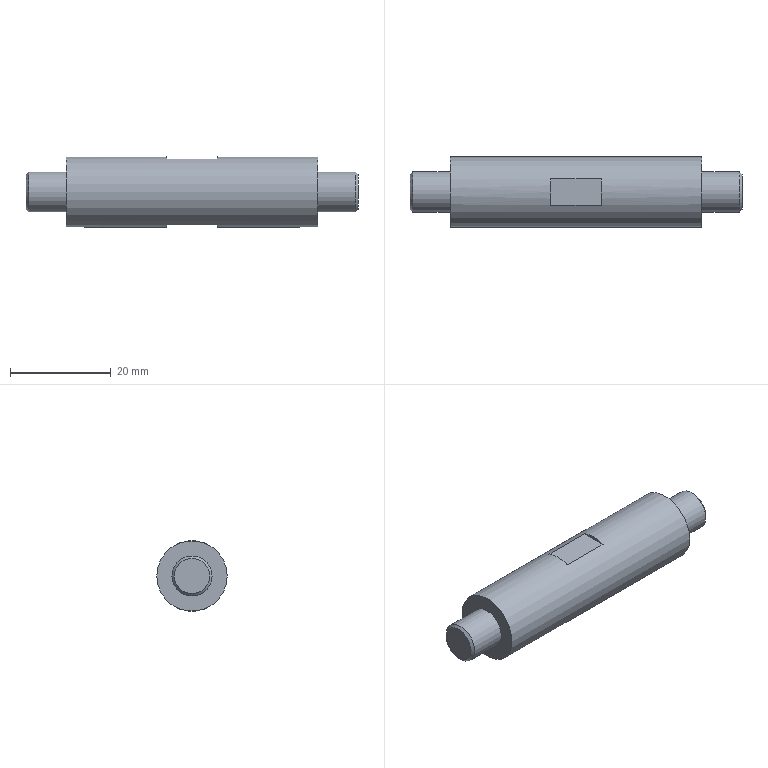Part | NX | features BREP 1 | 1 solid | 15 faces | box 66 x 14 x 14 mm | volume 8460 mm3 | plane 10 | cylinder 3 | cone 2 | commonest cylinder face diameters 8 x2 14 x1
STEP:
#1=CARTESIAN_POINT('',(-5.,-2.598,-6.5));
#2=VERTEX_POINT('',#1);
#3=CARTESIAN_POINT('',(-5.,2.598,-6.5));
#4=VERTEX_POINT('',#3);
#5=CARTESIAN_POINT('',(-5.,0.,0.));
#6=DIRECTION('',(1.,0.,0.));
#7=DIRECTION('',(0.,0.,1.));
#8=AXIS2_PLACEMENT_3D('',#5,#6,#7);
#9=CIRCLE('',#8,7.);
#10=EDGE_CURVE('',#2,#4,#9,.T.);
#11=ORIENTED_EDGE('',*,*,#10,.F.);
#12=CARTESIAN_POINT('',(5.,-2.598,-6.5));
#13=VERTEX_POINT('',#12);
#14=CARTESIAN_POINT('',(33.,-2.598,-6.5));
#15=DIRECTION('',(-1.,0.,0.));
#16=VECTOR('',#15,1000.);
#17=LINE('',#14,#16);
#18=EDGE_CURVE('',#13,#2,#17,.T.);
#19=ORIENTED_EDGE('',*,*,#18,.F.);
#20=CARTESIAN_POINT('',(5.,2.598,-6.5));
#21=VERTEX_POINT('',#20);
#22=CARTESIAN_POINT('',(5.,0.,0.));
#23=DIRECTION('',(1.,0.,0.));
#24=DIRECTION('',(0.,0.,1.));
#25=AXIS2_PLACEMENT_3D('',#22,#23,#24);
#26=CIRCLE('',#25,7.);
#27=EDGE_CURVE('',#13,#21,#26,.T.);
#28=ORIENTED_EDGE('',*,*,#27,.T.);
#29=CARTESIAN_POINT('',(33.,2.598,-6.5));
#30=DIRECTION('',(1.,0.,0.));
#31=VECTOR('',#30,1000.);
#32=LINE('',#29,#31);
#33=EDGE_CURVE('',#4,#21,#32,.T.);
#34=ORIENTED_EDGE('',*,*,#33,.F.);
#35=EDGE_LOOP('',(#11,#19,#28,#34));
#36=FACE_BOUND('',#35,.T.);
#37=CARTESIAN_POINT('',(-25.,7.,0.));
#38=VERTEX_POINT('',#37);
#39=CARTESIAN_POINT('',(-25.,0.,0.));
#40=DIRECTION('',(1.,0.,0.));
#41=DIRECTION('',(0.,1.,0.));
#42=AXIS2_PLACEMENT_3D('',#39,#40,#41);
#43=CIRCLE('',#42,7.);
#44=EDGE_CURVE('',#38,#38,#43,.T.);
#45=ORIENTED_EDGE('',*,*,#44,.T.);
#46=EDGE_LOOP('',(#45));
#47=FACE_BOUND('',#46,.T.);
#48=CARTESIAN_POINT('',(25.,7.,0.));
#49=VERTEX_POINT('',#48);
#50=CARTESIAN_POINT('',(25.,0.,0.));
#51=DIRECTION('',(1.,0.,0.));
#52=DIRECTION('',(0.,1.,0.));
#53=AXIS2_PLACEMENT_3D('',#50,#51,#52);
#54=CIRCLE('',#53,7.);
#55=EDGE_CURVE('',#49,#49,#54,.T.);
#56=ORIENTED_EDGE('',*,*,#55,.F.);
#57=EDGE_LOOP('',(#56));
#58=FACE_BOUND('',#57,.T.);
#59=CARTESIAN_POINT('',(-5.,-2.598,6.5));
#60=VERTEX_POINT('',#59);
#61=CARTESIAN_POINT('',(5.,-2.598,6.5));
#62=VERTEX_POINT('',#61);
#63=CARTESIAN_POINT('',(33.,-2.598,6.5));
#64=DIRECTION('',(1.,0.,0.));
#65=VECTOR('',#64,1000.);
#66=LINE('',#63,#65);
#67=EDGE_CURVE('',#60,#62,#66,.T.);
#68=ORIENTED_EDGE('',*,*,#67,.F.);
#69=CARTESIAN_POINT('',(-5.,2.598,6.5));
#70=VERTEX_POINT('',#69);
#71=CARTESIAN_POINT('',(-5.,0.,0.));
#72=DIRECTION('',(-1.,0.,0.));
#73=DIRECTION('',(0.,0.,-1.));
#74=AXIS2_PLACEMENT_3D('',#71,#72,#73);
#75=CIRCLE('',#74,7.);
#76=EDGE_CURVE('',#60,#70,#75,.T.);
#77=ORIENTED_EDGE('',*,*,#76,.T.);
#78=CARTESIAN_POINT('',(5.,2.598,6.5));
#79=VERTEX_POINT('',#78);
#80=CARTESIAN_POINT('',(33.,2.598,6.5));
#81=DIRECTION('',(-1.,0.,0.));
#82=VECTOR('',#81,1000.);
#83=LINE('',#80,#82);
#84=EDGE_CURVE('',#79,#70,#83,.T.);
#85=ORIENTED_EDGE('',*,*,#84,.F.);
#86=CARTESIAN_POINT('',(5.,0.,0.));
#87=DIRECTION('',(-1.,0.,0.));
#88=DIRECTION('',(0.,0.,-1.));
#89=AXIS2_PLACEMENT_3D('',#86,#87,#88);
#90=CIRCLE('',#89,7.);
#91=EDGE_CURVE('',#62,#79,#90,.T.);
#92=ORIENTED_EDGE('',*,*,#91,.F.);
#93=EDGE_LOOP('',(#68,#77,#85,#92));
#94=FACE_BOUND('',#93,.T.);
#95=CARTESIAN_POINT('',(33.,0.,0.));
#96=DIRECTION('',(1.,0.,0.));
#97=DIRECTION('',(0.,-1.,0.));
#98=AXIS2_PLACEMENT_3D('',#95,#96,#97);
#99=CYLINDRICAL_SURFACE('',#98,7.);
#100=ADVANCED_FACE('',(#36,#47,#58,#94),#99,.T.);
#101=CARTESIAN_POINT('',(33.,3.5,0.));
#102=VERTEX_POINT('',#101);
#103=CARTESIAN_POINT('',(33.,0.,0.));
#104=DIRECTION('',(1.,0.,0.));
#105=DIRECTION('',(0.,1.,0.));
#106=AXIS2_PLACEMENT_3D('',#103,#104,#105);
#107=CIRCLE('',#106,3.5);
#108=EDGE_CURVE('',#102,#102,#107,.T.);
#109=ORIENTED_EDGE('',*,*,#108,.T.);
#110=EDGE_LOOP('',(#109));
#111=FACE_BOUND('',#110,.T.);
#112=CARTESIAN_POINT('',(33.,4.,0.));
#113=DIRECTION('',(1.,0.,0.));
#114=DIRECTION('',(0.,-1.,0.));
#115=AXIS2_PLACEMENT_3D('',#112,#113,#114);
#116=PLANE('',#115);
#117=ADVANCED_FACE('',(#111),#116,.T.);
#118=CARTESIAN_POINT('',(-33.,-3.5,0.));
#119=VERTEX_POINT('',#118);
#120=CARTESIAN_POINT('',(-33.,0.,0.));
#121=DIRECTION('',(-1.,0.,0.));
#122=DIRECTION('',(0.,-1.,0.));
#123=AXIS2_PLACEMENT_3D('',#120,#121,#122);
#124=CIRCLE('',#123,3.5);
#125=EDGE_CURVE('',#119,#119,#124,.T.);
#126=ORIENTED_EDGE('',*,*,#125,.T.);
#127=EDGE_LOOP('',(#126));
#128=FACE_BOUND('',#127,.T.);
#129=CARTESIAN_POINT('',(-33.,0.,0.));
#130=DIRECTION('',(-1.,0.,0.));
#131=DIRECTION('',(0.,1.,0.));
#132=AXIS2_PLACEMENT_3D('',#129,#130,#131);
#133=PLANE('',#132);
#134=ADVANCED_FACE('',(#128),#133,.T.);
#135=CARTESIAN_POINT('',(-32.5,-4.,0.));
#136=VERTEX_POINT('',#135);
#137=CARTESIAN_POINT('',(-32.5,0.,0.));
#138=DIRECTION('',(1.,0.,0.));
#139=DIRECTION('',(0.,-1.,0.));
#140=AXIS2_PLACEMENT_3D('',#137,#138,#139);
#141=CIRCLE('',#140,4.);
#142=EDGE_CURVE('',#136,#136,#141,.T.);
#143=ORIENTED_EDGE('',*,*,#142,.T.);
#144=EDGE_LOOP('',(#143));
#145=FACE_BOUND('',#144,.T.);
#146=CARTESIAN_POINT('',(-25.,4.,0.));
#147=VERTEX_POINT('',#146);
#148=CARTESIAN_POINT('',(-25.,0.,0.));
#149=DIRECTION('',(1.,0.,0.));
#150=DIRECTION('',(0.,1.,0.));
#151=AXIS2_PLACEMENT_3D('',#148,#149,#150);
#152=CIRCLE('',#151,4.);
#153=EDGE_CURVE('',#147,#147,#152,.T.);
#154=ORIENTED_EDGE('',*,*,#153,.F.);
#155=EDGE_LOOP('',(#154));
#156=FACE_BOUND('',#155,.T.);
#157=CARTESIAN_POINT('',(33.,0.,0.));
#158=DIRECTION('',(1.,0.,0.));
#159=DIRECTION('',(0.,-1.,0.));
#160=AXIS2_PLACEMENT_3D('',#157,#158,#159);
#161=CYLINDRICAL_SURFACE('',#160,4.);
#162=ADVANCED_FACE('',(#145,#156),#161,.T.);
#163=ORIENTED_EDGE('',*,*,#153,.T.);
#164=EDGE_LOOP('',(#163));
#165=FACE_BOUND('',#164,.T.);
#166=ORIENTED_EDGE('',*,*,#44,.F.);
#167=EDGE_LOOP('',(#166));
#168=FACE_BOUND('',#167,.T.);
#169=CARTESIAN_POINT('',(-25.,4.,0.));
#170=DIRECTION('',(-1.,0.,0.));
#171=DIRECTION('',(0.,1.,0.));
#172=AXIS2_PLACEMENT_3D('',#169,#170,#171);
#173=PLANE('',#172);
#174=ADVANCED_FACE('',(#165,#168),#173,.T.);
#175=ORIENTED_EDGE('',*,*,#55,.T.);
#176=EDGE_LOOP('',(#175));
#177=FACE_BOUND('',#176,.T.);
#178=CARTESIAN_POINT('',(25.,4.,0.));
#179=VERTEX_POINT('',#178);
#180=CARTESIAN_POINT('',(25.,0.,0.));
#181=DIRECTION('',(1.,0.,0.));
#182=DIRECTION('',(0.,1.,0.));
#183=AXIS2_PLACEMENT_3D('',#180,#181,#182);
#184=CIRCLE('',#183,4.);
#185=EDGE_CURVE('',#179,#179,#184,.T.);
#186=ORIENTED_EDGE('',*,*,#185,.F.);
#187=EDGE_LOOP('',(#186));
#188=FACE_BOUND('',#187,.T.);
#189=CARTESIAN_POINT('',(25.,7.,0.));
#190=DIRECTION('',(1.,0.,0.));
#191=DIRECTION('',(0.,-1.,0.));
#192=AXIS2_PLACEMENT_3D('',#189,#190,#191);
#193=PLANE('',#192);
#194=ADVANCED_FACE('',(#177,#188),#193,.T.);
#195=CARTESIAN_POINT('',(32.5,4.,0.));
#196=VERTEX_POINT('',#195);
#197=CARTESIAN_POINT('',(32.5,0.,0.));
#198=DIRECTION('',(-1.,0.,0.));
#199=DIRECTION('',(0.,1.,0.));
#200=AXIS2_PLACEMENT_3D('',#197,#198,#199);
#201=CIRCLE('',#200,4.);
#202=EDGE_CURVE('',#196,#196,#201,.T.);
#203=ORIENTED_EDGE('',*,*,#202,.T.);
#204=EDGE_LOOP('',(#203));
#205=FACE_BOUND('',#204,.T.);
#206=ORIENTED_EDGE('',*,*,#185,.T.);
#207=EDGE_LOOP('',(#206));
#208=FACE_BOUND('',#207,.T.);
#209=CARTESIAN_POINT('',(33.,0.,0.));
#210=DIRECTION('',(1.,0.,0.));
#211=DIRECTION('',(0.,-1.,0.));
#212=AXIS2_PLACEMENT_3D('',#209,#210,#211);
#213=CYLINDRICAL_SURFACE('',#212,4.);
#214=ADVANCED_FACE('',(#205,#208),#213,.T.);
#215=ORIENTED_EDGE('',*,*,#202,.F.);
#216=EDGE_LOOP('',(#215));
#217=FACE_BOUND('',#216,.T.);
#218=ORIENTED_EDGE('',*,*,#108,.F.);
#219=EDGE_LOOP('',(#218));
#220=FACE_BOUND('',#219,.T.);
#221=CARTESIAN_POINT('',(33.,0.,0.));
#222=DIRECTION('',(-1.,0.,0.));
#223=DIRECTION('',(0.,1.,0.));
#224=AXIS2_PLACEMENT_3D('',#221,#222,#223);
#225=CONICAL_SURFACE('',#224,3.5,0.7854);
#226=ADVANCED_FACE('',(#217,#220),#225,.T.);
#227=ORIENTED_EDGE('',*,*,#125,.F.);
#228=EDGE_LOOP('',(#227));
#229=FACE_BOUND('',#228,.T.);
#230=ORIENTED_EDGE('',*,*,#142,.F.);
#231=EDGE_LOOP('',(#230));
#232=FACE_BOUND('',#231,.T.);
#233=CARTESIAN_POINT('',(-32.5,0.,0.));
#234=DIRECTION('',(1.,0.,0.));
#235=DIRECTION('',(0.,-1.,0.));
#236=AXIS2_PLACEMENT_3D('',#233,#234,#235);
#237=CONICAL_SURFACE('',#236,4.,0.7854);
#238=ADVANCED_FACE('',(#229,#232),#237,.T.);
#239=ORIENTED_EDGE('',*,*,#18,.T.);
#240=CARTESIAN_POINT('',(-5.,6.966,-6.5));
#241=DIRECTION('',(0.,-1.,0.));
#242=VECTOR('',#241,1000.);
#243=LINE('',#240,#242);
#244=EDGE_CURVE('',#4,#2,#243,.T.);
#245=ORIENTED_EDGE('',*,*,#244,.F.);
#246=ORIENTED_EDGE('',*,*,#33,.T.);
#247=CARTESIAN_POINT('',(5.,6.966,-6.5));
#248=DIRECTION('',(0.,-1.,0.));
#249=VECTOR('',#248,1000.);
#250=LINE('',#247,#249);
#251=EDGE_CURVE('',#21,#13,#250,.T.);
#252=ORIENTED_EDGE('',*,*,#251,.T.);
#253=EDGE_LOOP('',(#239,#245,#246,#252));
#254=FACE_BOUND('',#253,.T.);
#255=CARTESIAN_POINT('',(-5.,6.966,-6.5));
#256=DIRECTION('',(0.,0.,1.));
#257=DIRECTION('',(-1.,0.,0.));
#258=AXIS2_PLACEMENT_3D('',#255,#256,#257);
#259=PLANE('',#258);
#260=ADVANCED_FACE('',(#254),#259,.F.);
#261=ORIENTED_EDGE('',*,*,#10,.T.);
#262=ORIENTED_EDGE('',*,*,#244,.T.);
#263=EDGE_LOOP('',(#261,#262));
#264=FACE_BOUND('',#263,.T.);
#265=CARTESIAN_POINT('',(-5.,0.,0.));
#266=DIRECTION('',(-1.,0.,0.));
#267=DIRECTION('',(0.,0.,-1.));
#268=AXIS2_PLACEMENT_3D('',#265,#266,#267);
#269=PLANE('',#268);
#270=ADVANCED_FACE('',(#264),#269,.F.);
#271=ORIENTED_EDGE('',*,*,#251,.F.);
#272=ORIENTED_EDGE('',*,*,#27,.F.);
#273=EDGE_LOOP('',(#271,#272));
#274=FACE_BOUND('',#273,.T.);
#275=CARTESIAN_POINT('',(5.,0.,0.));
#276=DIRECTION('',(-1.,0.,0.));
#277=DIRECTION('',(0.,0.,-1.));
#278=AXIS2_PLACEMENT_3D('',#275,#276,#277);
#279=PLANE('',#278);
#280=ADVANCED_FACE('',(#274),#279,.T.);
#281=ORIENTED_EDGE('',*,*,#84,.T.);
#282=CARTESIAN_POINT('',(-5.,6.407,6.5));
#283=DIRECTION('',(0.,1.,0.));
#284=VECTOR('',#283,1000.);
#285=LINE('',#282,#284);
#286=EDGE_CURVE('',#60,#70,#285,.T.);
#287=ORIENTED_EDGE('',*,*,#286,.F.);
#288=ORIENTED_EDGE('',*,*,#67,.T.);
#289=CARTESIAN_POINT('',(5.,6.407,6.5));
#290=DIRECTION('',(0.,1.,0.));
#291=VECTOR('',#290,1000.);
#292=LINE('',#289,#291);
#293=EDGE_CURVE('',#62,#79,#292,.T.);
#294=ORIENTED_EDGE('',*,*,#293,.T.);
#295=EDGE_LOOP('',(#281,#287,#288,#294));
#296=FACE_BOUND('',#295,.T.);
#297=CARTESIAN_POINT('',(-5.,6.407,6.5));
#298=DIRECTION('',(0.,0.,-1.));
#299=DIRECTION('',(1.,0.,0.));
#300=AXIS2_PLACEMENT_3D('',#297,#298,#299);
#301=PLANE('',#300);
#302=ADVANCED_FACE('',(#296),#301,.F.);
#303=ORIENTED_EDGE('',*,*,#286,.T.);
#304=ORIENTED_EDGE('',*,*,#76,.F.);
#305=EDGE_LOOP('',(#303,#304));
#306=FACE_BOUND('',#305,.T.);
#307=CARTESIAN_POINT('',(-5.,0.,0.));
#308=DIRECTION('',(1.,0.,0.));
#309=DIRECTION('',(0.,0.,1.));
#310=AXIS2_PLACEMENT_3D('',#307,#308,#309);
#311=PLANE('',#310);
#312=ADVANCED_FACE('',(#306),#311,.T.);
#313=ORIENTED_EDGE('',*,*,#91,.T.);
#314=ORIENTED_EDGE('',*,*,#293,.F.);
#315=EDGE_LOOP('',(#313,#314));
#316=FACE_BOUND('',#315,.T.);
#317=CARTESIAN_POINT('',(5.,0.,0.));
#318=DIRECTION('',(1.,0.,0.));
#319=DIRECTION('',(0.,0.,1.));
#320=AXIS2_PLACEMENT_3D('',#317,#318,#319);
#321=PLANE('',#320);
#322=ADVANCED_FACE('',(#316),#321,.F.);
#323=CLOSED_SHELL('',(#100,#117,#134,#162,#174,#194,#214,#226,#238,#260,#270,#280,#302,#312,#322));
#324=MANIFOLD_SOLID_BREP('',#323);
#325=(LENGTH_UNIT()NAMED_UNIT(*)SI_UNIT(.MILLI.,.METRE.));
#326=UNCERTAINTY_MEASURE_WITH_UNIT(LENGTH_MEASURE(0.00001),#325,'','');
#327=(NAMED_UNIT(*)PLANE_ANGLE_UNIT()SI_UNIT($,.RADIAN.));
#328=(NAMED_UNIT(*)SI_UNIT($,.STERADIAN.)SOLID_ANGLE_UNIT());
#329=(GEOMETRIC_REPRESENTATION_CONTEXT(3)GLOBAL_UNCERTAINTY_ASSIGNED_CONTEXT((#326))GLOBAL_UNIT_ASSIGNED_CONTEXT((#325,#327,#328))REPRESENTATION_CONTEXT('',''));
#330=ADVANCED_BREP_SHAPE_REPRESENTATION('',(#324),#329);